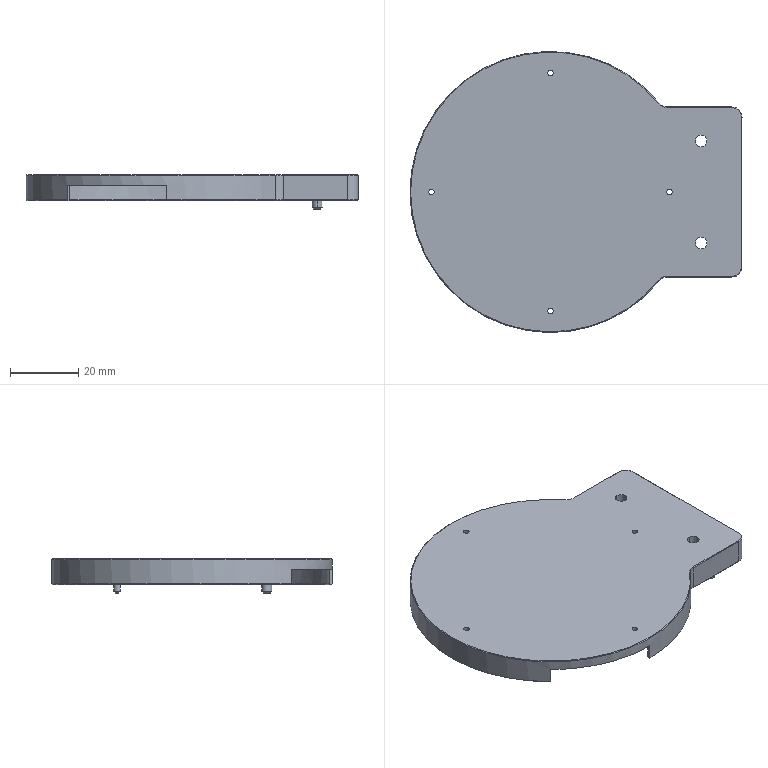NC program | NX | posted with a generic post | part box 97.6 x 82.6 x 10 mm
Lines 921 to 2560 of 4898:
(CAVITY_MILL_COPY , TOOL : D6)
N1840 T12 M6
N1842 G54
N1844 G17 G0 G90 X-18.675 Y-42.8 S9500 M3
N1846 G43 Z30. H12
N1848 Z1.
N1850 G94 G1 X-21. Z0.878 F1000.
N1852 Y-44.8 Z0.773
N1854 X-14. Z0.406
N1856 Y-42.8 Z0.302
N1858 X-21. Z-0.065
N1860 Y-44.8 Z-0.17
N1862 X-14. Z-0.537
N1864 Y-42.8 Z-0.642
N1866 X-21. Z-1.009
N1868 Y-44.8 Z-1.113
N1870 X-14. Z-1.48
N1872 Y-42.8 Z-1.585
N1874 X-21. Z-1.952
N1876 Y-44.8 Z-2.057
N1878 X-14. Z-2.424
N1880 Y-42.8 Z-2.528
N1882 X-21. Z-2.895
N1884 Y-44.8 Z-3.
N1886 X-14. F1500.
N1888 Y-42.8
N1890 X-21.
N1892 Y-44.8
N1894 G3 X-20.134 Y-44.3 R1.
N1896 G1 Z-2.
N1898 G0 X-14. Y-44.422
N1900 G1 Y-42.8 Z-2.085 F1000.
N1902 X-21. Z-2.452
N1904 Y-44.8 Z-2.557
N1906 X-14. Z-2.924
N1908 Y-42.8 Z-3.028
N1910 X-21. Z-3.395
N1912 Y-44.8 Z-3.5
N1914 X-14. F1500.
N1916 Y-42.8
N1918 X-21.
N1920 Y-44.8
N1922 G3 X-20.134 Y-44.3 R1.
N1924 G1 Z-2.5
N1926 G0 X-14. Y-44.422
N1928 G1 Y-42.8 Z-2.585 F1000.
N1930 X-21. Z-2.952
N1932 Y-44.8 Z-3.057
N1934 X-14. Z-3.424
N1936 Y-42.8 Z-3.528
N1938 X-21. Z-3.895
N1940 Y-44.8 Z-4.
N1942 X-14. F1500.
N1944 Y-42.8
N1946 X-21.
N1948 Y-44.8
N1950 G3 X-20.134 Y-44.3 R1.
N1952 G1 Z-3.
N1954 G0 X-14. Y-44.422
N1956 G1 Y-42.8 Z-3.085 F1000.
N1958 X-21. Z-3.452
N1960 Y-44.8 Z-3.557
N1962 X-14. Z-3.924
N1964 Y-42.8 Z-4.028
N1966 X-21. Z-4.395
N1968 Y-44.8 Z-4.5
N1970 X-14. F1500.
N1972 Y-42.8
N1974 X-21.
N1976 Y-44.8
N1978 G3 X-20.134 Y-44.3 R1.
N1980 G1 Z-3.5
N1982 G0 X-14. Y-44.422
N1984 G1 Y-42.8 Z-3.585 F1000.
N1986 X-21. Z-3.952
N1988 Y-44.8 Z-4.057
N1990 X-14. Z-4.424
N1992 Y-42.8 Z-4.528
N1994 X-21. Z-4.895
N1996 Y-44.8 Z-5.
N1998 X-14. F1500.
N2000 Y-42.8
N2002 X-21.
N2004 Y-44.8
N2006 G3 X-20.134 Y-44.3 R1.
N2008 G1 Z-4.
N2010 G0 X-14. Y-44.422
N2012 G1 Y-42.8 Z-4.085 F1000.
N2014 X-21. Z-4.452
N2016 Y-44.8 Z-4.557
N2018 X-14. Z-4.924
N2020 Y-42.8 Z-5.028
N2022 X-21. Z-5.395
N2024 Y-44.8 Z-5.5
N2026 X-14. F1500.
N2028 Y-42.8
N2030 X-21.
N2032 Y-44.8
N2034 G3 X-20.134 Y-44.3 R1.
N2036 G1 Z-4.5
N2038 G0 X-14. Y-44.423
N2040 G1 X-14.001 Y-42.8 Z-4.585 F1000.
N2042 X-21. Z-4.952
N2044 Y-44.8 Z-5.057
N2046 X-14. Z-5.424
N2048 X-14.001 Y-42.8 Z-5.528
N2050 X-21. Z-5.895
N2052 Y-44.8 Z-6.
N2054 X-14. F1500.
N2056 X-14.001 Y-42.8
N2058 X-21.
N2060 Y-44.8
N2062 G3 X-20.134 Y-44.3 R1.
N2064 G1 Z-5.
N2066 G0 X-14. Y-44.423
N2068 G1 X-14.001 Y-42.8 Z-5.085 F1000.
N2070 X-21. Z-5.452
N2072 Y-44.8 Z-5.557
N2074 X-14. Z-5.924
N2076 X-14.001 Y-42.8 Z-6.028
N2078 X-21. Z-6.395
N2080 Y-44.8 Z-6.5
N2082 X-14. F1500.
N2084 X-14.001 Y-42.8
N2086 X-21.
N2088 Y-44.8
N2090 G3 X-20.134 Y-44.3 R1.
N2092 G1 Z-5.5
N2094 G0 X-14. Y-44.423
N2096 G1 X-14.001 Y-42.8 Z-5.585 F1000.
N2098 X-21. Z-5.952
N2100 Y-44.8 Z-6.057
N2102 X-14. Z-6.424
N2104 X-14.001 Y-42.8 Z-6.528
N2106 X-21. Z-6.895
N2108 Y-44.8 Z-7.
N2110 X-14. F1500.
N2112 X-14.001 Y-42.8
N2114 X-21.
N2116 Y-44.8
N2118 G3 X-20.134 Y-44.3 R1.
N2120 G1 Z-6.
N2122 G0 X-14. Y-44.423
N2124 G1 X-14.001 Y-42.8 Z-6.085 F1000.
N2126 X-21. Z-6.452
N2128 Y-44.8 Z-6.557
N2130 X-14. Y-44.799 Z-6.924
N2132 X-14.001 Y-42.8 Z-7.028
N2134 X-21. Z-7.395
N2136 Y-44.8 Z-7.5
N2138 X-14. Y-44.799 F1500.
N2140 X-14.001 Y-42.8
N2142 X-21.
N2144 Y-44.8
N2146 G3 X-20.134 Y-44.3 R1.
N2148 G1 Z-6.5
N2150 G0 X-14. Y-44.424
N2152 G1 X-14.001 Y-42.8 Z-6.585 F1000.
N2154 X-20.999 Z-6.952
N2156 X-21. Y-44.8 Z-7.057
N2158 X-14. Y-44.799 Z-7.424
N2160 X-14.001 Y-42.8 Z-7.528
N2162 X-20.999 Z-7.895
N2164 X-21. Y-44.8 Z-8.
N2166 X-14. Y-44.799 F1500.
N2168 X-14.001 Y-42.8
N2170 X-20.999
N2172 X-21. Y-44.8
N2174 G3 X-20.134 Y-44.3 R1.
N2176 G1 Z-7.
N2178 G0 X-14. Y-44.425
N2180 G1 X-14.001 Y-42.8 Z-7.085 F1000.
N2182 X-20.999 Z-7.452
N2184 X-21. Y-44.8 Z-7.557
N2186 X-14. Y-44.799 Z-7.924
N2188 X-14.001 Y-42.8 Z-8.028
N2190 X-20.999 Z-8.395
N2192 X-21. Y-44.8 Z-8.5
N2194 X-14. Y-44.799 F1500.
N2196 X-14.001 Y-42.8
N2198 X-20.999
N2200 X-21. Y-44.8
N2202 G3 X-20.134 Y-44.3 R1.
N2204 G1 Z-7.5
N2206 G0 X-14. Y-44.426
N2208 G1 X-14.001 Y-42.8 Z-7.585 F1000.
N2210 X-20.999 Z-7.952
N2212 X-21. Y-44.8 Z-8.057
N2214 X-14. Y-44.799 Z-8.424
N2216 X-14.001 Y-42.8 Z-8.528
N2218 X-20.999 Z-8.895
N2220 X-21. Y-44.8 Z-9.
N2222 X-14. Y-44.799 F1500.
N2224 X-14.001 Y-42.8
N2226 X-20.999
N2228 X-21. Y-44.8
N2230 G3 X-20.134 Y-44.3 R1.
N2232 G1 Z-8.
N2234 G0 Z30.
N2236 X-5.8 Y-41.523
N2238 Z-2.
N2240 G1 Z-3. F1000.
N2242 X-6.5 Y-41.928
N2244 G3 X-7. Y-42.794 R1.
N2246 G1 Y-44.8 F1500.
N2248 X-4.994
N2250 G3 X-4.128 Y-44.3 R1.
N2252 G1 X-3.723 Y-43.6
N2254 Z-2.
N2256 G0 X-5.8 Y-41.523 Z-2.5
N2258 G1 Z-3.5 F1000.
N2260 X-6.5 Y-41.928
N2262 G3 X-7. Y-42.794 R1.
N2264 G1 Y-44.8 F1500.
N2266 X-4.994
N2268 G3 X-4.128 Y-44.3 R1.
N2270 G1 X-3.723 Y-43.6
N2272 Z-2.5
N2274 G0 X-5.8 Y-41.523 Z-3.
N2276 G1 Z-4. F1000.
N2278 X-6.5 Y-41.928
N2280 G3 X-7. Y-42.794 R1.
N2282 G1 Y-44.8 F1500.
N2284 X-4.994
N2286 G3 X-4.128 Y-44.3 R1.
N2288 G1 X-3.723 Y-43.6
N2290 Z-3.
N2292 G0 X-5.8 Y-41.523 Z-3.5
N2294 G1 Z-4.5 F1000.
N2296 X-6.5 Y-41.928
N2298 G3 X-7. Y-42.794 R1.
N2300 G1 Y-44.8 F1500.
N2302 X-4.994
N2304 G3 X-4.128 Y-44.3 R1.
N2306 G1 X-3.723 Y-43.6
N2308 Z-3.5
N2310 G0 X-5.8 Y-41.523 Z-4.
N2312 G1 Z-5. F1000.
N2314 X-6.5 Y-41.928
N2316 G3 X-7. Y-42.794 R1.
N2318 G1 Y-44.8 F1500.
N2320 X-4.994
N2322 G3 X-4.128 Y-44.3 R1.
N2324 G1 X-3.723 Y-43.6
N2326 Z-4.
N2328 G0 X-5.8 Y-41.523 Z-4.5
N2330 G1 Z-5.5 F1000.
N2332 X-6.5 Y-41.928
N2334 G3 X-7. Y-42.794 R1.
N2336 G1 Y-44.8 F1500.
N2338 X-4.994
N2340 G3 X-4.128 Y-44.3 R1.
N2342 G1 X-3.723 Y-43.6
N2344 Z-4.5
N2346 G0 X-5.8 Y-41.523 Z-5.
N2348 G1 Z-6. F1000.
N2350 X-6.5 Y-41.928
N2352 G3 X-7. Y-42.794 R1.
N2354 G1 Y-44.8 F1500.
N2356 X-4.994
N2358 G3 X-4.128 Y-44.3 R1.
N2360 G1 X-3.723 Y-43.6
N2362 Z-5.
N2364 G0 X-5.8 Y-41.523 Z-5.5
N2366 G1 Z-6.5 F1000.
N2368 X-6.5 Y-41.928
N2370 G3 X-7. Y-42.794 R1.
N2372 G1 Y-44.8 F1500.
N2374 X-4.994
N2376 G3 X-4.128 Y-44.3 R1.
N2378 G1 X-3.723 Y-43.6
N2380 Z-5.5
N2382 G0 X-5.8 Y-41.523 Z-6.
N2384 G1 Z-7. F1000.
N2386 X-6.5 Y-41.928
N2388 G3 X-7. Y-42.794 R1.
N2390 G1 Y-44.8 F1500.
N2392 X-4.994
N2394 G3 X-4.128 Y-44.3 R1.
N2396 G1 X-3.723 Y-43.6
N2398 Z-6.
N2400 G0 X-5.8 Y-41.523 Z-6.5
N2402 G1 Z-7.5 F1000.
N2404 X-6.5 Y-41.928
N2406 G3 X-7. Y-42.794 R1.
N2408 G1 Y-44.8 F1500.
N2410 X-4.994
N2412 G3 X-4.128 Y-44.3 R1.
N2414 G1 X-3.723 Y-43.6
N2416 Z-6.5
N2418 G0 X-5.8 Y-41.523 Z-7.
N2420 G1 Z-8. F1000.
N2422 X-6.5 Y-41.928
N2424 G3 X-7. Y-42.794 R1.
N2426 G1 Y-44.8 F1500.
N2428 X-4.994
N2430 G3 X-4.128 Y-44.3 R1.
N2432 G1 X-3.723 Y-43.6
N2434 Z-7.
N2436 G0 X-5.8 Y-41.523 Z-7.5
N2438 G1 Z-8.5 F1000.
N2440 X-6.5 Y-41.928
N2442 G3 X-7. Y-42.794 R1.
N2444 G1 Y-44.8 F1500.
N2446 X-4.994
N2448 G3 X-4.128 Y-44.3 R1.
N2450 G1 X-3.723 Y-43.6
N2452 Z-7.5
N2454 G0 X-5.8 Y-41.523 Z-8.
N2456 G1 Z-9. F1000.
N2458 X-6.5 Y-41.928
N2460 G3 X-7. Y-42.794 R1.
N2462 G1 Y-44.8 F1500.
N2464 X-4.994
N2466 G3 X-4.128 Y-44.3 R1.
N2468 G1 X-3.723 Y-43.6
N2470 Z-8.
N2472 G0 Z30.
N2474 X-3.641 Y-37.854
N2476 Z-2.
N2478 G1 Z-3. F1000.
N2480 X-3.96 Y-37.133
N2482 G3 X-4.767 Y-36.543 R1.
N2484 G2 X-7. Y-36.244 R44.3 F1500.
N2486 G1 Y-38.536
N2488 G3 X-6.5 Y-39.402 R1.
N2490 G1 X-5.8 Y-39.806
N2492 Z-2.
N2494 G0 X-3.641 Y-37.854 Z-2.5
N2496 G1 Z-3.5 F1000.
N2498 X-3.96 Y-37.133
N2500 G3 X-4.767 Y-36.543 R1.
N2502 G2 X-7. Y-36.244 R44.3 F1500.
N2504 G1 Y-38.536
N2506 G3 X-6.5 Y-39.402 R1.
N2508 G1 X-5.8 Y-39.806
N2510 Z-2.5
N2512 G0 X-3.641 Y-37.854 Z-3.
N2514 G1 Z-4. F1000.
N2516 X-3.96 Y-37.133
N2518 G3 X-4.767 Y-36.543 R1.
N2520 G2 X-7. Y-36.244 R44.3 F1500.
N2522 G1 Y-38.536
N2524 G3 X-6.5 Y-39.402 R1.
N2526 G1 X-5.8 Y-39.806
N2528 Z-3.
N2530 G0 X-3.641 Y-37.854 Z-3.5
N2532 G1 Z-4.5 F1000.
N2534 X-3.96 Y-37.133
N2536 G3 X-4.767 Y-36.543 R1.
N2538 G2 X-7. Y-36.244 R44.3 F1500.
N2540 G1 Y-38.536
N2542 G3 X-6.5 Y-39.402 R1.
N2544 G1 X-5.8 Y-39.806
N2546 Z-3.5
N2548 G0 X-3.641 Y-37.854 Z-4.
N2550 G1 Z-5. F1000.
N2552 X-3.96 Y-37.133
N2554 G3 X-4.767 Y-36.543 R1.
N2556 G2 X-7. Y-36.244 R44.3 F1500.
N2558 G1 Y-38.536
N2560 G3 X-6.5 Y-39.402 R1.
N2562 G1 X-5.8 Y-39.806
N2564 Z-4.
N2566 G0 X-3.641 Y-37.854 Z-4.5
N2568 G1 Z-5.5 F1000.
N2570 X-3.96 Y-37.133
N2572 G3 X-4.767 Y-36.543 R1.
N2574 G2 X-7. Y-36.244 R44.301 F1500.
N2576 G1 Y-38.536
N2578 G3 X-6.5 Y-39.402 R1.
N2580 G1 X-5.8 Y-39.806
N2582 Z-4.5
N2584 G0 X-3.641 Y-37.854 Z-5.
N2586 G1 Z-6. F1000.
N2588 X-3.96 Y-37.133
N2590 G3 X-4.767 Y-36.543 R1.
N2592 G2 X-7. Y-36.244 R44.301 F1500.
N2594 G1 Y-38.536
N2596 G3 X-6.5 Y-39.402 R1.
N2598 G1 X-5.8 Y-39.806
N2600 Z-5.
N2602 G0 X-3.641 Y-37.854 Z-5.5
N2604 G1 Z-6.5 F1000.
N2606 X-3.96 Y-37.133
N2608 G3 X-4.767 Y-36.543 R1.
N2610 G2 X-7. Y-36.244 R44.301 F1500.
N2612 G1 Y-38.536
N2614 G3 X-6.5 Y-39.402 R1.
N2616 G1 X-5.8 Y-39.806
N2618 Z-5.5
N2620 G0 X-3.641 Y-37.854 Z-6.
N2622 G1 Z-7. F1000.
N2624 X-3.96 Y-37.133
N2626 G3 X-4.767 Y-36.543 R1.
N2628 G2 X-7. Y-36.244 R44.301 F1500.
N2630 G1 Y-38.536
N2632 G3 X-6.5 Y-39.402 R1.
N2634 G1 X-5.8 Y-39.806
N2636 Z-6.
N2638 G0 X-3.641 Y-37.854 Z-6.5
N2640 G1 Z-7.5 F1000.
N2642 X-3.96 Y-37.133
N2644 G3 X-4.767 Y-36.543 R1.
N2646 G2 X-7. Y-36.244 R44.301 F1500.
N2648 G1 Y-38.536
N2650 G3 X-6.5 Y-39.402 R1.
N2652 G1 X-5.8 Y-39.806
N2654 Z-6.5
N2656 G0 X-3.641 Y-37.854 Z-7.
N2658 G1 Z-8. F1000.
N2660 X-3.96 Y-37.133
N2662 G3 X-4.767 Y-36.543 R1.
N2664 G2 X-7. Y-36.244 R44.301 F1500.
N2666 G1 Y-38.536
N2668 G3 X-6.5 Y-39.402 R1.
N2670 G1 X-5.8 Y-39.806
N2672 Z-7.
N2674 G0 X-3.641 Y-37.854 Z-7.5
N2676 G1 Z-8.5 F1000.
N2678 X-3.96 Y-37.133
N2680 G3 X-4.767 Y-36.543 R1.
N2682 G2 X-7. Y-36.245 R44.301 F1500.
N2684 G1 Y-38.536
N2686 G3 X-6.5 Y-39.402 R1.
N2688 G1 X-5.8 Y-39.806
N2690 Z-7.5
N2692 G0 X-3.641 Y-37.854 Z-8.
N2694 G1 Z-9. F1000.
N2696 X-3.96 Y-37.133
N2698 G3 X-4.767 Y-36.543 R1.
N2700 G2 X-7. Y-36.245 R44.301 F1500.
N2702 G1 Y-38.536
N2704 G3 X-6.5 Y-39.402 R1.
N2706 G1 X-5.8 Y-39.806
N2708 Z-8.
N2710 G0 Z30.
N2712 X-8.895 Y-27.487
N2714 Z-6.5
N2716 G1 Z-7.5 F1000.
N2718 X-8.64 Y-28.282
N2720 G3 X-7.9 Y-28.954 R1.
N2722 X-5.5 Y-29.392 R37.3 F1500.
N2724 G1 Y-27.5
N2726 G2 X-5.482 Y-27.055 R5.5
N2728 G3 X-5.91 Y-26.152 R1.
N2730 G1 X-6.471 Y-25.764
N2732 Z-6.5
N2734 G0 X-8.895 Y-27.487 Z-7.
N2736 G1 Z-8. F1000.
N2738 X-8.64 Y-28.282
N2740 G3 X-7.9 Y-28.954 R1.
N2742 X-5.5 Y-29.392 R37.3 F1500.
N2744 G1 Y-27.5
N2746 G2 X-5.482 Y-27.055 R5.5
N2748 G3 X-5.91 Y-26.152 R1.
N2750 G1 X-6.471 Y-25.764
N2752 Z-7.
N2754 G0 X-8.895 Y-27.487 Z-7.5
N2756 G1 Z-8.5 F1000.
N2758 X-8.64 Y-28.282
N2760 G3 X-7.9 Y-28.954 R1.
N2762 X-5.5 Y-29.392 R37.3 F1500.
N2764 G1 Y-27.5
N2766 G2 X-5.482 Y-27.055 R5.5
N2768 G3 X-5.91 Y-26.152 R1.
N2770 G1 X-6.471 Y-25.764
N2772 Z-7.5
N2774 G0 X-8.895 Y-27.487 Z-8.
N2776 G1 Z-9. F1000.
N2778 X-8.64 Y-28.282
N2780 G3 X-7.9 Y-28.954 R1.
N2782 X-5.5 Y-29.392 R37.3 F1500.
N2784 G1 Y-27.5
N2786 G2 X-5.482 Y-27.055 R5.5
N2788 G3 X-5.91 Y-26.152 R1.
N2790 G1 X-6.471 Y-25.764
N2792 Z-8.
N2794 G0 Z30.
N2796 X5.8 Y-39.806
N2798 Z-2.
N2800 G1 Z-3. F1000.
N2802 X6.5 Y-39.402
N2804 G3 X7. Y-38.536 R1.
N2806 G1 Y-36.243 F1500.
N2808 G2 X4.767 Y-36.543 R44.3
N2810 G3 X3.96 Y-37.133 R1.
N2812 G1 X3.641 Y-37.854
N2814 Z-2.
N2816 G0 X5.8 Y-39.806 Z-2.5
N2818 G1 Z-3.5 F1000.
N2820 X6.5 Y-39.402
N2822 G3 X7. Y-38.536 R1.
N2824 G1 Y-36.243 F1500.
N2826 G2 X4.767 Y-36.543 R44.3
N2828 G3 X3.959 Y-37.133 R1.
N2830 G1 X3.641 Y-37.854
N2832 Z-2.5
N2834 G0 X5.8 Y-39.806 Z-3.
N2836 G1 Z-4. F1000.
N2838 X6.5 Y-39.402
N2840 G3 X7. Y-38.536 R1.
N2842 G1 Y-36.243 F1500.
N2844 G2 X4.767 Y-36.543 R44.3
N2846 G3 X3.959 Y-37.133 R1.
N2848 G1 X3.641 Y-37.854
N2850 Z-3.
N2852 G0 X5.8 Y-39.806 Z-3.5
N2854 G1 Z-4.5 F1000.
N2856 X6.5 Y-39.402
N2858 G3 X7. Y-38.536 R1.
N2860 G1 Y-36.243 F1500.
N2862 G2 X4.766 Y-36.543 R44.3
N2864 G3 X3.959 Y-37.133 R1.
N2866 G1 X3.641 Y-37.854
N2868 Z-3.5
N2870 G0 X5.8 Y-39.806 Z-4.
N2872 G1 Z-5. F1000.
N2874 X6.5 Y-39.402
N2876 G3 X7. Y-38.536 R1.
N2878 G1 Y-36.243 F1500.
N2880 G2 X4.766 Y-36.543 R44.3
N2882 G3 X3.959 Y-37.133 R1.
N2884 G1 X3.641 Y-37.854
N2886 Z-4.
N2888 G0 X5.8 Y-39.807 Z-4.5
N2890 G1 Z-5.5 F1000.
N2892 X6.5 Y-39.402
N2894 G3 X7. Y-38.536 R1.
N2896 G1 Y-36.243 F1500.
N2898 G2 X4.766 Y-36.543 R44.3
N2900 G3 X3.959 Y-37.133 R1.
N2902 G1 X3.641 Y-37.854
N2904 Z-4.5
N2906 G0 X5.8 Y-39.807 Z-5.
N2908 G1 Z-6. F1000.
N2910 X6.5 Y-39.403
N2912 G3 X7. Y-38.537 R1.
N2914 G1 Y-36.243 F1500.
N2916 G2 X4.766 Y-36.543 R44.3
N2918 G3 X3.959 Y-37.133 R1.
N2920 G1 X3.641 Y-37.854
N2922 Z-5.
N2924 G0 X5.8 Y-39.807 Z-5.5
N2926 G1 Z-6.5 F1000.
N2928 X6.5 Y-39.403
N2930 G3 X7. Y-38.537 R1.
N2932 G1 Y-36.243 F1500.
N2934 G2 X4.766 Y-36.543 R44.3
N2936 G3 X3.959 Y-37.133 R1.
N2938 G1 X3.64 Y-37.854
N2940 Z-5.5
N2942 G0 X5.8 Y-39.807 Z-6.
N2944 G1 Z-7. F1000.
N2946 X6.5 Y-39.403
N2948 G3 X7. Y-38.537 R1.
N2950 G1 Y-36.243 F1500.
N2952 G2 X4.766 Y-36.543 R44.3
N2954 G3 X3.959 Y-37.133 R1.
N2956 G1 X3.64 Y-37.854
N2958 Z-6.
N2960 G0 X5.8 Y-39.807 Z-6.5
N2962 G1 Z-7.5 F1000.
N2964 X6.5 Y-39.403
N2966 G3 X7. Y-38.537 R1.
N2968 G1 Y-36.243 F1500.
N2970 G2 X4.766 Y-36.543 R44.3
N2972 G3 X3.959 Y-37.133 R1.
N2974 G1 X3.64 Y-37.854
N2976 Z-6.5
N2978 G0 X5.8 Y-39.807 Z-7.
N2980 G1 Z-8. F1000.
N2982 X6.5 Y-39.403
N2984 G3 X7. Y-38.537 R1.
N2986 G1 Y-36.243 F1500.
N2988 G2 X4.766 Y-36.543 R44.3
N2990 G3 X3.958 Y-37.133 R1.
N2992 G1 X3.64 Y-37.854
N2994 Z-7.
N2996 G0 X5.8 Y-39.807 Z-7.5
N2998 G1 Z-8.5 F1000.
N3000 X6.5 Y-39.403
N3002 G3 X7. Y-38.537 R1.
N3004 G1 Y-36.243 F1500.
N3006 G2 X4.765 Y-36.543 R44.3
N3008 G3 X3.958 Y-37.133 R1.
N3010 G1 X3.64 Y-37.854
N3012 Z-7.5
N3014 G0 X5.8 Y-39.807 Z-8.
N3016 G1 Z-9. F1000.
N3018 X6.5 Y-39.403
N3020 G3 X7. Y-38.537 R1.
N3022 G1 Y-36.243 F1500.
N3024 G2 X4.765 Y-36.543 R44.3
N3026 G3 X3.958 Y-37.133 R1.
N3028 G1 X3.64 Y-37.854
N3030 Z-8.
N3032 G0 Z30.
N3034 X3.723 Y-43.6
N3036 Z-2.
N3038 G1 Z-3. F1000.
N3040 X4.128 Y-44.3
N3042 G3 X4.994 Y-44.8 R1.
N3044 G1 X7. F1500.
N3046 Y-42.794
N3048 G3 X6.5 Y-41.928 R1.
N3050 G1 X5.8 Y-41.523
N3052 Z-2.
N3054 G0 X3.723 Y-43.6 Z-2.5
N3056 G1 Z-3.5 F1000.
N3058 X4.128 Y-44.3
N3060 G3 X4.994 Y-44.8 R1.
N3062 G1 X7. F1500.
N3064 Y-42.794
N3066 G3 X6.5 Y-41.928 R1.
N3068 G1 X5.8 Y-41.523
N3070 Z-2.5
N3072 G0 X3.723 Y-43.6 Z-3.
N3074 G1 Z-4. F1000.
N3076 X4.128 Y-44.3
N3078 G3 X4.994 Y-44.8 R1.
N3080 G1 X7. F1500.
N3082 Y-42.794
N3084 G3 X6.5 Y-41.928 R1.
N3086 G1 X5.8 Y-41.523
N3088 Z-3.
N3090 G0 X3.723 Y-43.6 Z-3.5
N3092 G1 Z-4.5 F1000.
N3094 X4.128 Y-44.3
N3096 G3 X4.994 Y-44.8 R1.
N3098 G1 X7. F1500.
N3100 Y-42.794
N3102 G3 X6.5 Y-41.928 R1.
N3104 G1 X5.8 Y-41.523
N3106 Z-3.5
N3108 G0 X3.723 Y-43.6 Z-4.
N3110 G1 Z-5. F1000.
N3112 X4.128 Y-44.3
N3114 G3 X4.994 Y-44.8 R1.
N3116 G1 X7. F1500.
N3118 Y-42.794
N3120 G3 X6.5 Y-41.928 R1.
N3122 G1 X5.8 Y-41.523
N3124 Z-4.
N3126 G0 X3.723 Y-43.6 Z-4.5
N3128 G1 Z-5.5 F1000.
N3130 X4.128 Y-44.3
N3132 G3 X4.994 Y-44.8 R1.
N3134 G1 X7. F1500.
N3136 Y-42.794
N3138 G3 X6.5 Y-41.928 R1.
N3140 G1 X5.8 Y-41.523
N3142 Z-4.5
N3144 G0 X3.723 Y-43.6 Z-5.
N3146 G1 Z-6. F1000.
N3148 X4.128 Y-44.3
N3150 G3 X4.994 Y-44.8 R1.
N3152 G1 X7. F1500.
N3154 Y-42.794
N3156 G3 X6.5 Y-41.928 R1.
N3158 G1 X5.8 Y-41.523
N3160 Z-5.
N3162 G0 X3.723 Y-43.6 Z-5.5
N3164 G1 Z-6.5 F1000.
N3166 X4.128 Y-44.3
N3168 G3 X4.994 Y-44.8 R1.
N3170 G1 X7. F1500.
N3172 Y-42.794
N3174 G3 X6.5 Y-41.928 R1.
N3176 G1 X5.8 Y-41.523
N3178 Z-5.5
N3180 G0 X3.723 Y-43.6 Z-6.
N3182 G1 Z-7. F1000.
N3184 X4.128 Y-44.3
N3186 G3 X4.994 Y-44.8 R1.
N3188 G1 X7. F1500.
N3190 Y-42.794
N3192 G3 X6.5 Y-41.928 R1.
N3194 G1 X5.8 Y-41.523
N3196 Z-6.
N3198 G0 X3.723 Y-43.6 Z-6.5
N3200 G1 Z-7.5 F1000.
N3202 X4.128 Y-44.3
N3204 G3 X4.994 Y-44.8 R1.
N3206 G1 X7. Y-44.799 F1500.
N3208 Y-42.794
N3210 G3 X6.5 Y-41.928 R1.
N3212 G1 X5.8 Y-41.523
N3214 Z-6.5
N3216 G0 X3.723 Y-43.6 Z-7.
N3218 G1 Z-8. F1000.
N3220 X4.128 Y-44.3
N3222 G3 X4.994 Y-44.8 R1.
N3224 G1 X7. Y-44.799 F1500.
N3226 Y-42.794
N3228 G3 X6.5 Y-41.928 R1.
N3230 G1 X5.8 Y-41.523
N3232 Z-7.
N3234 G0 X3.723 Y-43.6 Z-7.5
N3236 G1 Z-8.5 F1000.
N3238 X4.128 Y-44.3
N3240 G3 X4.994 Y-44.8 R1.
N3242 G1 X7. Y-44.799 F1500.
N3244 Y-42.794
N3246 G3 X6.5 Y-41.928 R1.
N3248 G1 X5.8 Y-41.523
N3250 Z-7.5
N3252 G0 X3.723 Y-43.6 Z-8.
N3254 G1 Z-9. F1000.
N3256 X4.128 Y-44.3
N3258 G3 X4.994 Y-44.8 R1.
N3260 G1 X7. Y-44.799 F1500.
N3262 Y-42.794
N3264 G3 X6.5 Y-41.928 R1.
N3266 G1 X5.8 Y-41.523
N3268 Z-8.
N3270 G0 Z30.
N3272 X16.324 Y-42.8
N3274 Z1.
N3276 G1 X14. Z0.878 F1000.
N3278 Y-44.8 Z0.773
N3280 X21. Z0.407
N3282 Y-42.8 Z0.302
N3284 X14. Z-0.065
N3286 Y-44.8 Z-0.17
N3288 X21. Z-0.537
N3290 Y-42.8 Z-0.642
N3292 X14. Z-1.009
N3294 Y-44.8 Z-1.113
N3296 X21. Z-1.48
N3298 Y-42.8 Z-1.585
N3300 X14. Z-1.952
N3302 Y-44.8 Z-2.057
N3304 X21. Z-2.424
N3306 Y-42.8 Z-2.528
N3308 X14. Z-2.895
N3310 Y-44.8 Z-3.
N3312 X21. F1500.
N3314 Y-42.8
N3316 X14.
N3318 Y-44.8
N3320 G3 X14.866 Y-44.3 R1.
N3322 G1 Z-2.
N3324 G0 X21. Y-44.422
N3326 G1 Y-42.8 Z-2.085 F1000.
N3328 X14. Z-2.452
N3330 Y-44.8 Z-2.557
N3332 X21. Z-2.924
N3334 Y-42.8 Z-3.028
N3336 X14. Z-3.395
N3338 Y-44.8 Z-3.5
N3340 X21. F1500.
N3342 Y-42.8
N3344 X14.
N3346 Y-44.8
N3348 G3 X14.866 Y-44.3 R1.
N3350 G1 Z-2.5
N3352 G0 X21. Y-44.422
N3354 G1 Y-42.8 Z-2.585 F1000.
N3356 X14. Z-2.952
N3358 Y-44.8 Z-3.057
N3360 X21. Z-3.424
N3362 Y-42.8 Z-3.528
N3364 X14. Z-3.895
N3366 Y-44.8 Z-4.
N3368 X21. F1500.
N3370 Y-42.8
N3372 X14.
N3374 Y-44.8
N3376 G3 X14.866 Y-44.3 R1.
N3378 G1 Z-3.
N3380 G0 X21. Y-44.422
N3382 G1 Y-42.8 Z-3.085 F1000.
N3384 X14. Z-3.452
N3386 Y-44.8 Z-3.557
N3388 X21. Z-3.924
N3390 Y-42.8 Z-4.028
N3392 X14. Z-4.395
N3394 Y-44.8 Z-4.5
N3396 X21. F1500.
N3398 Y-42.8
N3400 X14.
N3402 Y-44.8
N3404 G3 X14.866 Y-44.3 R1.
N3406 G1 Z-3.5
N3408 G0 X21. Y-44.422
N3410 G1 Y-42.8 Z-3.585 F1000.
N3412 X14. Z-3.952
N3414 Y-44.8 Z-4.057
N3416 X21. Z-4.424
N3418 Y-42.8 Z-4.528
N3420 X14. Z-4.895
N3422 Y-44.8 Z-5.
N3424 X21. F1500.
N3426 Y-42.8
N3428 X14.
N3430 Y-44.8
N3432 G3 X14.866 Y-44.3 R1.
N3434 G1 Z-4.
N3436 G0 X21. Y-44.422
N3438 G1 Y-42.8 Z-4.085 F1000.
N3440 X14. Z-4.452
N3442 Y-44.8 Z-4.557
N3444 X21. Z-4.924
N3446 Y-42.8 Z-5.028
N3448 X14. Z-5.395
N3450 Y-44.8 Z-5.5
N3452 X21. F1500.
N3454 Y-42.8
N3456 X14.
N3458 Y-44.8
N3460 G3 X14.866 Y-44.3 R1.
N3462 G1 Z-4.5
N3464 G0 X21. Y-44.422
N3466 G1 Y-42.8 Z-4.585 F1000.
N3468 X14. Z-4.952
N3470 Y-44.8 Z-5.057
N3472 X21. Z-5.424
N3474 Y-42.8 Z-5.528
N3476 X14. Z-5.895
N3478 Y-44.8 Z-6.
N3480 X21. F1500.
N3482 Y-42.8
N3484 X14.
N3486 Y-44.8
N3488 G3 X14.866 Y-44.3 R1.
N3490 G1 Z-5.
N3492 G0 X21. Y-44.422
N3494 G1 Y-42.8 Z-5.085 F1000.
N3496 X14. Z-5.452
N3498 Y-44.8 Z-5.557
N3500 X21. Z-5.924
N3502 Y-42.8 Z-6.028
N3504 X14. Z-6.395
N3506 Y-44.8 Z-6.5
N3508 X21. F1500.
N3510 Y-42.8
N3512 X14.
N3514 Y-44.8
N3516 G3 X14.866 Y-44.3 R1.
N3518 G1 Z-5.5
N3520 G0 X21. Y-44.422
N3522 G1 Y-42.8 Z-5.585 F1000.
N3524 X14. Z-5.952
N3526 Y-44.8 Z-6.057
N3528 X21. Z-6.424
N3530 Y-42.8 Z-6.528
N3532 X14. Z-6.895
N3534 Y-44.8 Z-7.
N3536 X21. F1500.
N3538 Y-42.8
N3540 X14.
N3542 Y-44.8
N3544 G3 X14.866 Y-44.3 R1.
N3546 G1 Z-6.
N3548 G0 X21. Y-44.422
N3550 G1 Y-42.8 Z-6.085 F1000.
N3552 X14. Z-6.452
N3554 Y-44.8 Z-6.557
N3556 X21. Z-6.924
N3558 Y-42.8 Z-7.028
N3560 X14. Z-7.395
N3562 Y-44.8 Z-7.5
N3564 X21. F1500.
N3566 Y-42.8
N3568 X14.
N3570 Y-44.8
N3572 G3 X14.866 Y-44.3 R1.
N3574 G1 Z-6.5
N3576 G0 X21. Y-44.423
N3578 G1 Y-42.8 Z-6.585 F1000.
N3580 X14.001 Z-6.952
N3582 X14. Y-44.8 Z-7.057
N3584 X21. Z-7.424
N3586 Y-42.8 Z-7.528
N3588 X14.001 Z-7.895
N3590 X14. Y-44.8 Z-8.
N3592 X21. F1500.
N3594 Y-42.8
N3596 X14.001
N3598 X14. Y-44.8
N3600 G3 X14.866 Y-44.3 R1.
N3602 G1 Z-7.
N3604 G0 X21. Y-44.424
N3606 G1 Y-42.8 Z-7.085 F1000.
N3608 X14.001 Z-7.452
N3610 X14. Y-44.8 Z-7.557
N3612 X21. Z-7.924
N3614 Y-42.8 Z-8.028
N3616 X14.001 Z-8.395
N3618 X14. Y-44.8 Z-8.5
N3620 X21. F1500.
N3622 Y-42.8
N3624 X14.001
N3626 X14. Y-44.8
N3628 G3 X14.866 Y-44.3 R1.
N3630 G1 Z-7.5
N3632 G0 X21. Y-44.425
N3634 G1 Y-42.8 Z-7.585 F1000.
N3636 X14.001 Z-7.952
N3638 X14. Y-44.8 Z-8.057
N3640 X21. Z-8.424
N3642 Y-42.8 Z-8.528
N3644 X14.001 Z-8.895
N3646 X14. Y-44.8 Z-9.
N3648 X21. F1500.
N3650 Y-42.8
N3652 X14.001
N3654 X14. Y-44.8
N3656 G3 X14.866 Y-44.3 R1.
N3658 G1 Z-8.
N3660 G0 Z30.
N3662 X6.471 Y-25.764
N3664 Z-6.5
N3666 G1 Z-7.5 F1000.
N3668 X5.91 Y-26.152
N3670 G3 X5.482 Y-27.055 R1.
N3672 G2 X5.5 Y-27.5 R5.5 F1500.
N3674 G1 Y-29.392
N3676 G3 X7.9 Y-28.954 R37.3
N3678 X8.64 Y-28.282 R1.
N3680 G1 X8.895 Y-27.487
N3682 Z-6.5
N3684 G0 X6.471 Y-25.764 Z-7.
N3686 G1 Z-8. F1000.
N3688 X5.91 Y-26.152
N3690 G3 X5.482 Y-27.055 R1.
N3692 G2 X5.5 Y-27.5 R5.5 F1500.
N3694 G1 Y-29.392
N3696 G3 X7.9 Y-28.954 R37.3
N3698 X8.64 Y-28.282 R1.
N3700 G1 X8.895 Y-27.487
N3702 Z-7.
N3704 G0 X6.471 Y-25.764 Z-7.5
N3706 G1 Z-8.5 F1000.
N3708 X5.91 Y-26.152
N3710 G3 X5.482 Y-27.055 R1.
N3712 G2 X5.5 Y-27.5 R5.5 F1500.
N3714 G1 Y-29.392
N3716 G3 X7.9 Y-28.954 R37.3
N3718 X8.64 Y-28.282 R1.
N3720 G1 X8.895 Y-27.487
N3722 Z-7.5
N3724 G0 X6.471 Y-25.764 Z-8.
N3726 G1 Z-9. F1000.
N3728 X5.91 Y-26.152
N3730 G3 X5.482 Y-27.055 R1.
N3732 G2 X5.5 Y-27.5 R5.5 F1500.
N3734 G1 Y-29.392
N3736 G3 X7.9 Y-28.954 R37.3
N3738 X8.64 Y-28.282 R1.
N3740 G1 X8.895 Y-27.487
N3742 Z-8.
N3744 G0 Z30.
N3746 X34.987 Y-1.394
N3748 Z-6.5
N3750 G1 Z-7.5 F1000.
N3752 X35.782 Y-1.14
N3754 G3 X36.454 Y-0.399 R1.
N3756 X36.892 Y2. R37.3 F1500.
N3758 G1 X35.
N3760 G2 X34.555 Y2.018 R5.5
N3762 G3 X33.652 Y1.59 R1.
N3764 G1 X33.264 Y1.029
N3766 Z-6.5
N3768 G0 X34.987 Y-1.394 Z-7.
N3770 G1 Z-8. F1000.
N3772 X35.782 Y-1.14
N3774 G3 X36.454 Y-0.399 R1.
N3776 X36.892 Y2. R37.3 F1500.
N3778 G1 X35.
N3780 G2 X34.555 Y2.018 R5.5
N3782 G3 X33.652 Y1.59 R1.
N3784 G1 X33.264 Y1.029
N3786 Z-7.
N3788 G0 X34.987 Y-1.394 Z-7.5
N3790 G1 Z-8.5 F1000.
N3792 X35.782 Y-1.14
N3794 G3 X36.454 Y-0.399 R1.
N3796 X36.892 Y2. R37.3 F1500.
N3798 G1 X35.
N3800 G2 X34.555 Y2.018 R5.5
N3802 G3 X33.652 Y1.59 R1.
N3804 G1 X33.264 Y1.029
N3806 Z-7.5
N3808 G0 X34.987 Y-1.394 Z-8.
N3810 G1 Z-9. F1000.
N3812 X35.782 Y-1.14
N3814 G3 X36.454 Y-0.399 R1.
N3816 X36.892 Y2. R37.3 F1500.
N3818 G1 X35.
N3820 G2 X34.555 Y2.018 R5.5
N3822 G3 X33.652 Y1.59 R1.
N3824 G1 X33.264 Y1.029
N3826 Z-8.
N3828 G0 Z30.
N3830 Y13.971
N3832 Z-6.5
N3834 G1 Z-7.5 F1000.
N3836 X33.652 Y13.41
N3838 G3 X34.555 Y12.982 R1.
N3840 G2 X35. Y13. R5.5 F1500.
N3842 G1 X36.892
N3844 G3 X36.454 Y15.4 R37.3
N3846 X35.782 Y16.14 R1.
N3848 G1 X34.987 Y16.395
N3850 Z-6.5
N3852 G0 X33.264 Y13.971 Z-7.
N3854 G1 Z-8. F1000.
N3856 X33.652 Y13.41
N3858 G3 X34.555 Y12.982 R1.
N3860 G2 X35. Y13. R5.5 F1500.
N3862 G1 X36.892 Y13.001
N3864 G3 X36.454 Y15.4 R37.3
N3866 X35.782 Y16.14 R1.
N3868 G1 X34.987 Y16.395
N3870 Z-7.
N3872 G0 X33.264 Y13.971 Z-7.5
N3874 G1 Z-8.5 F1000.
N3876 X33.652 Y13.41
N3878 G3 X34.555 Y12.982 R1.
N3880 G2 X35. Y13. R5.5 F1500.
N3882 G1 X36.892 Y13.001
N3884 G3 X36.454 Y15.4 R37.3
N3886 X35.782 Y16.14 R1.
N3888 G1 X34.987 Y16.395
N3890 Z-7.5
N3892 G0 X33.264 Y13.971 Z-8.
N3894 G1 Z-9. F1000.
N3896 X33.652 Y13.41
N3898 G3 X34.555 Y12.982 R1.
N3900 G2 X35. Y13. R5.5 F1500.
N3902 G1 X36.892 Y13.001
N3904 G3 X36.454 Y15.4 R37.3
N3906 X35.782 Y16.14 R1.
N3908 G1 X34.987 Y16.395
N3910 Z-8.
N3912 G0 Z30.
N3914 X8.895 Y42.487
N3916 Z-6.5
N3918 G1 Z-7.5 F1000.
N3920 X8.64 Y43.282
N3922 G3 X7.9 Y43.954 R1.
N3924 X5.5 Y44.392 R37.3 F1500.
N3926 G1 Y42.5
N3928 G2 X5.482 Y42.055 R5.5
N3930 G3 X5.91 Y41.152 R1.
N3932 G1 X6.471 Y40.764
N3934 Z-6.5
N3936 G0 X8.895 Y42.487 Z-7.
N3938 G1 Z-8. F1000.
N3940 X8.64 Y43.282
N3942 G3 X7.9 Y43.954 R1.
N3944 X5.5 Y44.392 R37.3 F1500.
N3946 G1 Y42.5
N3948 G2 X5.482 Y42.055 R5.5
N3950 G3 X5.91 Y41.152 R1.
N3952 G1 X6.471 Y40.764
N3954 Z-7.
N3956 G0 X8.895 Y42.487 Z-7.5
N3958 G1 Z-8.5 F1000.
N3960 X8.64 Y43.282
N3962 G3 X7.9 Y43.954 R1.
N3964 X5.5 Y44.392 R37.3 F1500.
N3966 G1 Y42.5
N3968 G2 X5.482 Y42.055 R5.5
N3970 G3 X5.91 Y41.152 R1.
N3972 G1 X6.471 Y40.764
N3974 Z-7.5
N3976 G0 X8.895 Y42.487 Z-8.
N3978 G1 Z-9. F1000.
N3980 X8.64 Y43.282
N3982 G3 X7.9 Y43.954 R1.
N3984 X5.5 Y44.392 R37.3 F1500.
N3986 G1 Y42.5
N3988 G2 X5.482 Y42.055 R5.5
N3990 G3 X5.91 Y41.152 R1.
N3992 G1 X6.471 Y40.764
N3994 Z-8.
N3996 G0 Z30.
N3998 X-6.471
N4000 Z-6.5
N4002 G1 Z-7.5 F1000.
N4004 X-5.91 Y41.152
N4006 G3 X-5.482 Y42.055 R1.
N4008 G2 X-5.5 Y42.5 R5.5 F1500.
N4010 G1 Y44.392
N4012 G3 X-7.9 Y43.954 R37.3
N4014 X-8.64 Y43.282 R1.
N4016 G1 X-8.895 Y42.487
N4018 Z-6.5
N4020 G0 X-6.471 Y40.764 Z-7.
N4022 G1 Z-8. F1000.
N4024 X-5.91 Y41.152
N4026 G3 X-5.482 Y42.055 R1.
N4028 G2 X-5.5 Y42.5 R5.5 F1500.
N4030 G1 Y44.392
N4032 G3 X-7.9 Y43.954 R37.3
N4034 X-8.64 Y43.282 R1.
N4036 G1 X-8.895 Y42.487
N4038 Z-7.
N4040 G0 X-6.471 Y40.764 Z-7.5
N4042 G1 Z-8.5 F1000.
N4044 X-5.91 Y41.152
N4046 G3 X-5.482 Y42.055 R1.
N4048 G2 X-5.5 Y42.5 R5.5 F1500.
N4050 G1 Y44.392
N4052 G3 X-7.9 Y43.954 R37.3
N4054 X-8.64 Y43.282 R1.
N4056 G1 X-8.895 Y42.487
N4058 Z-7.5
N4060 G0 X-6.471 Y40.764 Z-8.
N4062 G1 Z-9. F1000.
N4064 X-5.91 Y41.152
N4066 G3 X-5.482 Y42.055 R1.
N4068 G2 X-5.5 Y42.5 R5.5 F1500.
N4070 G1 Y44.392
N4072 G3 X-7.9 Y43.954 R37.3
N4074 X-8.64 Y43.282 R1.
N4076 G1 X-8.895 Y42.487
N4078 Z-8.
N4080 G0 Z30.
N4082 X-34.987 Y16.395
N4084 Z-6.5
N4086 G1 Z-7.5 F1000.
N4088 X-35.782 Y16.14
N4090 G3 X-36.454 Y15.4 R1.
N4092 X-36.892 Y13. R37.3 F1500.
N4094 G1 X-35.
N4096 G2 X-34.555 Y12.982 R5.5
N4098 G3 X-33.652 Y13.41 R1.
N4100 G1 X-33.264 Y13.971
N4102 Z-6.5
N4104 G0 X-34.987 Y16.395 Z-7.
N4106 G1 Z-8. F1000.
N4108 X-35.782 Y16.14
N4110 G3 X-36.454 Y15.4 R1.
N4112 X-36.892 Y13. R37.3 F1500.
N4114 G1 X-35.
N4116 G2 X-34.555 Y12.982 R5.5
N4118 G3 X-33.652 Y13.41 R1.
N4120 G1 X-33.264 Y13.971
N4122 Z-7.
N4124 G0 X-34.987 Y16.395 Z-7.5
N4126 G1 Z-8.5 F1000.
N4128 X-35.782 Y16.14
N4130 G3 X-36.454 Y15.4 R1.
N4132 X-36.892 Y13. R37.3 F1500.
N4134 G1 X-35.
N4136 G2 X-34.555 Y12.982 R5.5
N4138 G3 X-33.652 Y13.41 R1.
N4140 G1 X-33.264 Y13.971
N4142 Z-7.5
N4144 G0 X-34.987 Y16.395 Z-8.
N4146 G1 Z-9. F1000.
N4148 X-35.782 Y16.14
N4150 G3 X-36.454 Y15.4 R1.
N4152 X-36.892 Y13. R37.3 F1500.
N4154 G1 X-35.
N4156 G2 X-34.555 Y12.982 R5.5
N4158 G3 X-33.652 Y13.41 R1.
N4160 G1 X-33.264 Y13.971
N4162 Z-8.
N4164 G0 Z30.
N4166 Y1.029
N4168 Z-6.5
N4170 G1 Z-7.5 F1000.
N4172 X-33.652 Y1.59
N4174 G3 X-34.555 Y2.018 R1.
N4176 G2 X-35. Y2. R5.5 F1500.
N4178 G1 X-36.892
N4180 G3 X-36.454 Y-0.4 R37.3
N4182 X-35.782 Y-1.14 R1.
N4184 G1 X-34.987 Y-1.395
N4186 Z-6.5
N4188 G0 X-33.264 Y1.029 Z-7.
N4190 G1 Z-8. F1000.
N4192 X-33.652 Y1.59
N4194 G3 X-34.555 Y2.018 R1.
N4196 G2 X-35. Y2. R5.5 F1500.
N4198 G1 X-36.892
N4200 G3 X-36.454 Y-0.4 R37.3
N4202 X-35.782 Y-1.14 R1.
N4204 G1 X-34.987 Y-1.395
N4206 Z-7.
N4208 G0 X-33.264 Y1.029 Z-7.5
N4210 G1 Z-8.5 F1000.
N4212 X-33.652 Y1.59
N4214 G3 X-34.555 Y2.018 R1.
N4216 G2 X-35. Y2. R5.5 F1500.
N4218 G1 X-36.892
N4220 G3 X-36.454 Y-0.4 R37.3
N4222 X-35.782 Y-1.14 R1.
N4224 G1 X-34.987 Y-1.395
N4226 Z-7.5
N4228 G0 X-33.264 Y1.029 Z-8.
N4230 G1 Z-9. F1000.
N4232 X-33.652 Y1.59
N4234 G3 X-34.555 Y2.018 R1.
N4236 G2 X-35. Y2. R5.5 F1500.
N4238 G1 X-36.892
N4240 G3 X-36.454 Y-0.4 R37.3
N4242 X-35.782 Y-1.14 R1.
N4244 G1 X-34.987 Y-1.395
N4246 Z-8.
N4248 G0 Z30.
(FLOOR_WALL , TOOL : D6)
N4250 X-4.399 Y-42.6
N4252 Z-1.4
N4254 G1 X-0.293 Z-2.5 F1100.
N4256 X12.244
N4258 G2 X10.69 Y-37.755 R11.35
N4260 X-11.182 Y-37.637 R46.5
N4262 X-12.83 Y-42.6 R10.85
N4264 G1 X-0.293
N4266 Y-45.6
N4268 X21.8
N4270 Y-45.148
N4272 G2 X14.294 Y-33.585 R8.35
N4274 X-14.947 Y-33.353 R43.5
N4276 X-21.8 Y-44.647 R7.85
N4278 G1 Y-45.6
N4280 X-0.293
N4282 Y-48.6
N4284 X22.
N4286 G3 X24.8 Y-45.8 R2.8
N4288 G1 Y-41.359
N4290 G2 X24.8 Y-32.241 R-5.35
N4292 G1 X24.486 Y-32.752
N4294 G2 X26.048 Y-39.286 R4.75
N4296 X24.486 Y-32.752 R-4.75
N4298 G1 X24.8 Y-32.241
N4300 Y-26.829
N4302 G2 X25.977 Y-24.349 R3.2
N4304 G3 X41.1 Y7.5 R41.1
N4306 G1 X40.498
N4308 G2 X28.636 Y36.136 R-40.5
N4310 G1 X29.062 Y36.562
N4312 G3 X-25.977 Y-24.349 R-41.1
N4314 G2 X-24.8 Y-26.829 R3.2
N4316 G1 Y-32.84
N4318 G2 X-24.8 Y-40.76 R-4.85
N4320 G1 X-24.454 Y-40.27
N4322 G2 X-25.47 Y-34.346 R4.25
N4324 X-24.454 Y-40.27 R-4.25
N4326 G1 X-24.8 Y-40.76
N4328 Y-45.8
N4330 G3 X-22. Y-48.6 R2.8
N4332 G1 X-0.293
N4334 Y-51.6
N4336 X22.
N4338 G3 X27.8 Y-45.8 R5.8
N4340 G1 Y-26.829
N4342 X27.799 Y-26.768
N4344 X27.826 Y-26.712
N4346 X27.874 Y-26.674
N4348 G3 X44.1 Y7.5 R44.1
N4350 G1 Y10.501
N4352 X37.498 Y10.498
N4354 Y7.5
N4356 G2 X26.515 Y34.015 R-37.5
N4358 G1 X28.636 Y31.894
N4360 X33.305 Y36.562
N4362 X31.183 Y38.683
N4364 G3 X-27.874 Y-26.674 R-44.1
N4366 G1 X-27.826 Y-26.712
N4368 X-27.799 Y-26.768
N4370 X-27.8 Y-26.829
N4372 Y-45.8
N4374 G3 X-22. Y-51.6 R5.8
N4376 G1 X-0.293
N4378 G2 X0.166 Y-51.814 R0.6
N4380 G1 Z-1.5
N4382 G0 Z30.
N4384 X22.662 Y-41.706
N4386 Z-1.5
N4388 G1 Z-2.5
N4390 X22.46 Y-41.464
N4392 G3 X22. Y-41.25 R0.6
N4394 G2 X17.55 Y-36.8 R4.45
N4396 X22. Y-41.25 R-4.45
N4398 G3 X21.54 Y-41.464 R0.6
N4400 G1 X21.338 Y-41.706
N4402 Z-1.5
N4404 G0 Z30.
N4406 X-21.342 Y-41.201
N4408 Z-1.5
N4410 G1 Z-2.5
N4412 X-21.54 Y-40.964
N4414 G3 X-22. Y-40.75 R0.6
N4416 G2 X-25.95 Y-36.8 R3.95
N4418 X-22. Y-40.75 R-3.95
N4420 G3 X-22.46 Y-40.964 R0.6
N4422 G1 X-22.658 Y-41.201
N4424 Z-1.5
N4426 G0 Z30.
N4428 X0.975 Y-26.489
N4430 Z-5.9
N4432 G1 X1.434 Y-26.48 Z-6.023
N4434 X2.257 Y-26.425 Z-6.244
N4436 X2.161 Y-26.223 Z-6.304
N4438 X1.801 Y-25.751 Z-6.463
N4440 X1.34 Y-25.378 Z-6.622
N4442 X0.804 Y-25.122 Z-6.781
N4444 X0.224 Y-25. Z-6.94
N4446 X0. Z-7.
N4448 G3 X-2.257 Y-26.425 R2.5
N4450 X2.257 Y-26.425 R34.
N4452 X0. Y-25. R2.5
N4454 G1 Y-22.
N4456 G3 X-5.5 Y-27.5 R5.5
N4458 G1 Y-29.092
N4460 X-5.458 Y-29.095
N4462 G3 X5.458 Y-29.095 R37.
N4464 G1 X5.5 Y-29.092
N4466 Y-27.5
N4468 G3 X0. Y-22. R5.5
N4470 G2 X-0.46 Y-21.786 R0.6
N4472 G1 Z-6.
N4474 G0 Z30.
N4476 X-5.925 Y-29.112
N4478 Z-6.
N4480 G1 Z-7.
N4482 G3 X-5.502 Y-29.392 R0.6
N4484 X5.502 Y-29.392 R37.3
N4486 X5.925 Y-29.112 R0.6
N4488 G1 Z-6.
N4490 G0 Z30.
N4492 X1.986 Y7.04
N4494 Z-8.
N4496 G1 Z-9.
N4498 G3 X2.2 Y7.5 R0.6
N4500 G2 X2.279 Y9.779 R32.8
N4502 X-2.279 Y9.779 R32.8
N4504 X-2.279 Y5.221 R32.8
N4506 X2.279 Y5.221 R32.8
N4508 X2.2 Y7.5 R32.8
N4510 G1 X5.2
N4512 G2 X5.762 Y13.262 R29.8
N4514 X-5.762 Y13.262 R29.8
N4516 X-5.762 Y1.738 R29.8
N4518 X5.762 Y1.738 R29.8
N4520 X5.2 Y7.5 R29.8
N4522 G1 X8.2
N4524 G2 X10.229 Y17.729 R26.8
N4526 X-10.229 Y17.729 R26.8
N4528 X-10.229 Y-2.729 R26.8
N4530 X10.229 Y-2.729 R26.8
N4532 X8.2 Y7.5 R26.8
N4534 G1 X11.2
N4536 G2 X14.565 Y19.701 R23.8
N4538 G3 X12.201 Y22.065 R19.
N4540 G2 X-12.201 Y22.065 R23.8
N4542 G3 X-14.565 Y19.701 R19.
N4544 G2 X-14.565 Y-4.701 R23.8
N4546 G3 X-12.201 Y-7.065 R19.
N4548 G2 X12.201 Y-7.065 R23.8
N4550 G3 X14.565 Y-4.701 R19.
N4552 G2 X11.2 Y7.5 R23.8
N4554 G1 X14.2
N4556 G2 X18.234 Y19.81 R20.8
N4558 G3 X12.31 Y25.734 R22.
N4560 G2 X-12.31 Y25.734 R20.8
N4562 G3 X-18.234 Y19.81 R22.
N4564 G2 X-18.234 Y-4.81 R20.8
N4566 G3 X-12.31 Y-10.734 R22.
N4568 G2 X12.31 Y-10.734 R20.8
N4570 G3 X18.234 Y-4.81 R22.
N4572 G2 X14.2 Y7.5 R20.8
N4574 G1 X17.2
N4576 G2 X21.902 Y19.554 R17.8
N4578 G3 X12.054 Y29.402 R25.
N4580 G2 X-12.054 Y29.402 R17.8
N4582 G3 X-21.902 Y19.554 R25.
N4584 G2 X-21.902 Y-4.554 R17.8
N4586 G3 X-12.054 Y-14.402 R25.
N4588 G2 X12.054 Y-14.402 R17.8
N4590 G3 X21.902 Y-4.554 R25.
N4592 G2 X17.2 Y7.5 R17.8
N4594 G1 X20.2
N4596 G2 X25.571 Y18.908 R14.8
N4598 G3 X11.408 Y33.071 R28.
N4600 G2 X-11.408 Y33.071 R14.8
N4602 G3 X-25.571 Y18.908 R28.
N4604 G2 X-25.571 Y-3.908 R14.8
N4606 G3 X-11.408 Y-18.071 R28.
N4608 G2 X11.408 Y-18.071 R14.8
N4610 G3 X25.571 Y-3.908 R28.
N4612 G2 X20.2 Y7.5 R14.8
N4614 G1 X23.2
N4616 G2 X29.239 Y17.798 R11.8
N4618 G3 X10.298 Y36.739 R31.
N4620 G2 X-10.298 Y36.739 R11.8
N4622 G3 X-29.239 Y17.798 R31.
N4624 G2 X-29.239 Y-2.798 R11.8
N4626 G3 X-10.298 Y-21.739 R31.
N4628 G2 X10.298 Y-21.739 R11.8
N4630 G3 X29.239 Y-2.798 R31.
N4632 G2 X23.2 Y7.5 R11.8
N4634 G1 X26.2
N4636 G2 X32.908 Y16.048 R8.8
N4638 G3 X8.548 Y40.408 R34.
N4640 G2 X-8.548 Y40.408 R8.8
N4642 G3 X-32.908 Y16.048 R34.
N4644 G2 X-32.908 Y-1.048 R8.8
N4646 G3 X-8.548 Y-25.408 R34.
N4648 G2 X8.548 Y-25.408 R8.8
N4650 G3 X32.908 Y-1.048 R34.
N4652 G2 X26.2 Y7.5 R8.8
N4654 G1 X29.2
N4656 G2 X35. Y13.3 R5.8
N4658 G1 X36.543
N4660 G3 X5.8 Y44.043 R37.
N4662 G1 Y42.5
N4664 G2 X0. Y36.7 R5.8
N4666 X-5.8 Y42.5 R5.8
N4668 G1 Y44.043
N4670 G3 X-36.543 Y13.3 R37.
N4672 G1 X-35.
N4674 G2 X-29.2 Y7.5 R5.8
N4676 X-35. Y1.7 R5.8
N4678 G1 X-36.543
N4680 G3 X-5.8 Y-29.043 R37.
N4682 G1 Y-27.5
N4684 G2 X0. Y-21.7 R5.8
N4686 X5.8 Y-27.5 R5.8
N4688 G1 Y-29.043
N4690 G3 X36.543 Y1.7 R37.
N4692 G1 X35.
N4694 G2 X29.2 Y7.5 R5.8
N4696 G1 X29.286 Y7.04
N4698 G3 X29.5 Y7.5 R0.6
N4700 G2 X35. Y13. R5.5
N4702 G1 X36.892
N4704 G3 X5.5 Y44.392 R37.3
N4706 G1 Y42.5
N4708 G2 X0. Y37. R5.5
N4710 X-5.5 Y42.5 R5.5
N4712 G1 Y44.392
N4714 G3 X-36.892 Y13. R37.3
N4716 G1 X-35.
N4718 G2 X-29.5 Y7.5 R5.5
N4720 X-35. Y2. R5.5
N4722 G1 X-36.892
N4724 G3 X-5.5 Y-29.392 R37.3
N4726 G1 Y-27.5
N4728 G2 X0. Y-22. R5.5
N4730 X5.5 Y-27.5 R5.5
N4732 G1 Y-29.392
N4734 G3 X36.892 Y2. R37.3
N4736 G1 X35.
N4738 G2 X29.5 Y7.5 R5.5
N4740 G3 X29.286 Y7.96 R0.6
N4742 G1 Z-8.
N4744 G0 Z30.
N4746 X17.04 Y-44.286
N4748 Z-8.
N4750 G1 Z-9.
N4752 G3 X17.5 Y-44.5 R0.6
N4754 G1 X20.7
N4756 Y-43.1
N4758 X14.3
N4760 Y-44.5
N4762 X17.5
N4764 X17.04 Y-44.586
N4766 G3 X17.5 Y-44.8 R0.6
N4768 G1 X21.
N4770 Y-42.8
N4772 X14.
N4774 Y-44.8
N4776 X17.5
N4778 G3 X17.96 Y-44.586 R0.6
N4780 G1 Z-8.
N4782 G0 Z30.
N4784 X0.46 Y-40.314
N4786 Z-8.
N4788 G1 Z-9.
N4790 G3 X0. Y-40.1 R0.6
N4792 G2 X-3.7 Y-39.956 R47.6
N4794 G1 Y-41.5
N4796 X3.7
N4798 Y-39.956
N4800 G2 X0. Y-40.1 R47.6
N4802 G1 Y-37.1
N4804 G2 X-6.7 Y-36.594 R44.6
N4806 G1 Y-44.5
N4808 X6.7
N4810 Y-36.594
N4812 G2 X0. Y-37.1 R44.6
N4814 G1 X0.46 Y-37.014
N4816 G3 X0. Y-36.8 R0.6
N4818 G2 X-7. Y-36.243 R44.3
N4820 G1 Y-44.8
N4822 X7.
N4824 Y-36.243
N4826 G2 X0. Y-36.8 R44.3
N4828 G3 X-0.46 Y-37.014 R0.6
N4830 G1 Z-8.
N4832 G0 Z30.
N4834 X-17.04 Y-43.314
N4836 Z-8.
N4838 G1 Z-9.
N4840 G3 X-17.5 Y-43.1 R0.6
N4842 G1 X-20.7
N4844 Y-44.5
N4846 X-14.3
N4848 Y-43.1
N4850 X-17.5
N4852 X-17.04 Y-43.014
N4854 G3 X-17.5 Y-42.8 R0.6
N4856 G1 X-21.
N4858 Y-44.8
N4860 X-14.
N4862 Y-42.8
N4864 X-17.5
N4866 G3 X-17.96 Y-43.014 R0.6
N4868 G1 Z-8.
N4870 G0 Z30.
N4872 X-33.989 Y6.525
N4874 Z-5.9
N4876 G1 X-33.98 Y6.066 Z-6.023
N4878 X-33.925 Y5.243 Z-6.244
N4880 X-33.723 Y5.339 Z-6.304
N4882 X-33.251 Y5.699 Z-6.463
N4884 X-32.878 Y6.16 Z-6.622
N4886 X-32.622 Y6.696 Z-6.781
N4888 X-32.5 Y7.276 Z-6.94
N4890 Y7.5 Z-7.
N4892 G3 X-33.925 Y9.757 R2.5
N4894 X-33.925 Y5.243 R34.
N4896 X-32.5 Y7.5 R2.5
N4898 G1 X-29.5
N4900 G3 X-35. Y13. R5.5
N4902 G1 X-36.592
N4904 X-36.595 Y12.958
N4906 G3 X-36.595 Y2.042 R37.
N4908 G1 X-36.592 Y2.
N4910 X-35.
N4912 G3 X-29.5 Y7.5 R5.5
N4914 G2 X-29.286 Y7.96 R0.6
N4916 G1 Z-6.
N4918 G0 Z30.
N4920 X-36.612 Y13.425
N4922 Z-6.
N4924 G1 Z-7.
N4926 G3 X-36.892 Y13.002 R0.6
N4928 X-36.892 Y1.997 R37.3
N4930 X-36.612 Y1.575 R0.6
N4932 G1 Z-6.
N4934 G0 Z30.
N4936 X-0.975 Y41.489
N4938 Z-5.9
N4940 G1 X-1.434 Y41.48 Z-6.023
N4942 X-2.257 Y41.425 Z-6.244
N4944 X-2.161 Y41.223 Z-6.304
N4946 X-1.801 Y40.751 Z-6.463
N4948 X-1.34 Y40.378 Z-6.622
N4950 X-0.804 Y40.122 Z-6.781
N4952 X-0.224 Y40. Z-6.94
N4954 X0. Z-7.
N4956 G3 X2.257 Y41.425 R2.5
N4958 X-2.257 Y41.425 R34.
N4960 X0. Y40. R2.5
N4962 G1 Y37.
N4964 G3 X5.5 Y42.5 R5.5
N4966 G1 Y44.092
N4968 X5.458 Y44.095
N4970 G3 X-5.458 Y44.095 R37.
N4972 G1 X-5.5 Y44.092
N4974 Y42.5
N4976 G3 X0. Y37. R5.5
N4978 G2 X0.46 Y36.786 R0.6
N4980 G1 Z-6.
N4982 G0 Z30.
N4984 X5.925 Y44.112
N4986 Z-6.
N4988 G1 Z-7.
N4990 G3 X5.503 Y44.392 R0.6
N4992 X-5.503 Y44.392 R37.3
N4994 X-5.926 Y44.112 R0.6
N4996 G1 Z-6.
N4998 G0 Z30.
N5000 X39.534 Y19.44
N5002 Z-5.9
N5004 G1 X39.189 Y20.566 Z-6.215
N5006 X38.504 Y22.465 Z-6.756
N5008 X38.156 Y23.305 Z-7.
N5010 G3 X33.317 Y31.907 R41.3
N5012 G1 X32.601 Y31.191
N5014 G2 X39.805 Y13.8 R40.3
N5016 G1 X40.817
N5018 G3 X38.156 Y23.305 R41.3
N5020 G1 X40.928 Y24.453
N5022 G3 X33.571 Y36.404 R44.3
N5024 G1 X28.709 Y31.542
N5026 X28.655 Y31.487
N5028 X28.582 Y31.466
N5030 G2 X36.892 Y13. R37.3
N5032 G1 X35.
N5034 G3 X32.8 Y12.541 R5.5
N5036 G1 X34. Y9.791
N5038 G3 X33.925 Y5.243 R2.5
N5040 X34. Y7.5 R34.
N5042 G1 Y9.791
N5044 X32.8 Y12.541
N5046 G3 X35. Y2. R5.5
N5048 G1 X36.592
N5050 X36.595 Y2.042
N5052 G3 X37. Y7.5 R37.
N5054 G1 Y10.5
N5056 G2 X37.3 Y10.8 R0.3
N5058 G1 X44.177
N5060 G3 X40.928 Y24.453 R44.3
N5062 G2 X40.95 Y24.96 R0.6
N5064 G1 Z-6.
N5066 G0 Z30.
N5068 X33.851 Y36.805
N5070 Z-6.
N5072 G1 Z-7.
N5074 G3 X33.374 Y36.632 R0.6
N5076 G1 X28.496 Y31.754
N5078 X26.986 Y33.264
N5080 G3 X26.509 Y33.438 R0.6
N5082 G1 Z-6.
N5084 G0 Z30.
N5086 X36.612 Y1.575
N5088 Z-6.
N5090 G1 Z-7.
N5092 G3 X36.892 Y1.998 R0.6
N5094 X37.3 Y7.5 R37.3
N5096 G1 Y10.5
N5098 X44.198
N5100 G3 X44.658 Y10.714 R0.6
N5102 G1 Z-6.
N5104 G0 Z30.
N5106 M5